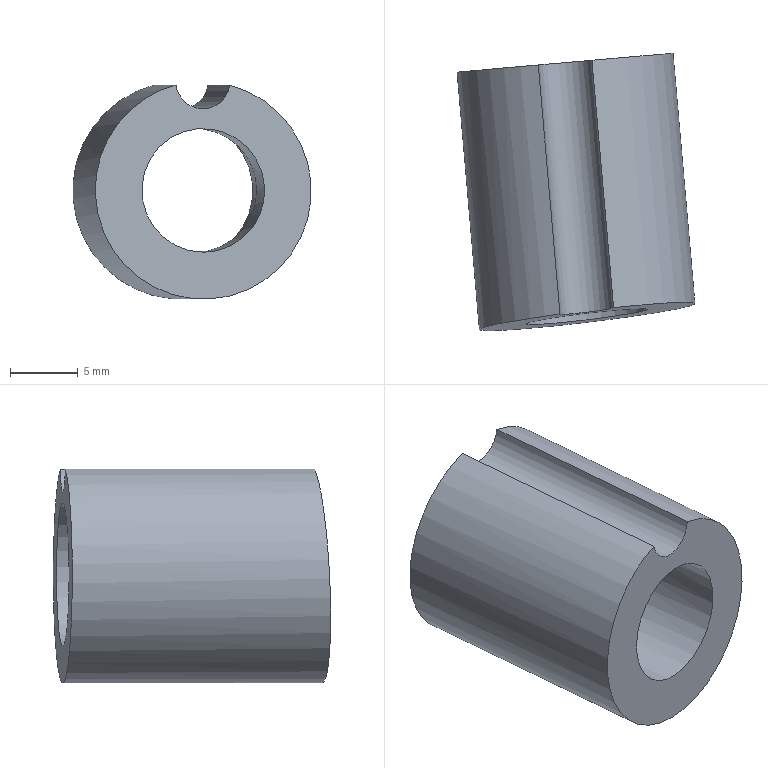Part | NX | features EKSD 16-20-9.100 2 | 1 solid | 7 faces | box 17.55 x 20.406 x 15.75 mm | volume 2161 mm3 | cylinder 4 | plane 3 | commonest cylinder face diameters 4 x1 9.1 x1 10.6 x1 16 x1
STEP:
#1=CARTESIAN_POINT('',(754.985,-30.446,-34.724));
#2=VERTEX_POINT('',#1);
#3=CARTESIAN_POINT('',(758.938,-30.1,-34.724));
#4=VERTEX_POINT('',#3);
#5=CARTESIAN_POINT('',(756.962,-30.273,-34.474));
#6=DIRECTION('',(0.08716,-0.9962,0.));
#7=DIRECTION('',(0.9962,0.08716,0.));
#8=AXIS2_PLACEMENT_3D('',#5,#6,#7);
#9=CIRCLE('',#8,2.);
#10=EDGE_CURVE('',#2,#4,#9,.T.);
#11=ORIENTED_EDGE('',*,*,#10,.T.);
#12=CARTESIAN_POINT('',(756.962,-30.273,-42.474));
#13=DIRECTION('',(0.08716,-0.9962,0.));
#14=DIRECTION('',(0.9962,0.08716,0.));
#15=AXIS2_PLACEMENT_3D('',#12,#13,#14);
#16=CIRCLE('',#15,8.);
#17=EDGE_CURVE('',#2,#4,#16,.T.);
#18=ORIENTED_EDGE('',*,*,#17,.F.);
#19=EDGE_LOOP('',(#11,#18));
#20=FACE_BOUND('',#19,.T.);
#21=CARTESIAN_POINT('',(751.682,-30.735,-42.474));
#22=VERTEX_POINT('',#21);
#23=CARTESIAN_POINT('',(756.962,-30.273,-42.474));
#24=DIRECTION('',(-0.08716,0.9962,0.));
#25=DIRECTION('',(-0.9962,-0.08716,0.));
#26=AXIS2_PLACEMENT_3D('',#23,#24,#25);
#27=CIRCLE('',#26,5.3);
#28=EDGE_CURVE('',#22,#22,#27,.T.);
#29=ORIENTED_EDGE('',*,*,#28,.F.);
#30=EDGE_LOOP('',(#29));
#31=FACE_BOUND('',#30,.T.);
#32=CARTESIAN_POINT('',(756.962,-30.273,-42.474));
#33=DIRECTION('',(-0.08716,0.9962,0.));
#34=DIRECTION('',(-0.9962,-0.08716,0.));
#35=AXIS2_PLACEMENT_3D('',#32,#33,#34);
#36=PLANE('',#35);
#37=ADVANCED_FACE('',(#20,#31),#36,.T.);
#38=CARTESIAN_POINT('',(760.531,-48.309,-34.724));
#39=VERTEX_POINT('',#38);
#40=CARTESIAN_POINT('',(756.589,-48.784,-34.724));
#41=VERTEX_POINT('',#40);
#42=CARTESIAN_POINT('',(758.559,-48.534,-34.474));
#43=DIRECTION('',(-0.1195,0.9915,-0.05097));
#44=DIRECTION('',(0.5313,0.1073,0.8404));
#45=AXIS2_PLACEMENT_3D('',#42,#43,#44);
#46=ELLIPSE('',#45,2.004,2.);
#47=EDGE_CURVE('',#39,#41,#46,.T.);
#48=ORIENTED_EDGE('',*,*,#47,.T.);
#49=CARTESIAN_POINT('',(758.595,-48.941,-42.474));
#50=DIRECTION('',(-0.1195,0.9915,-0.05097));
#51=DIRECTION('',(0.5313,0.1073,0.8404));
#52=AXIS2_PLACEMENT_3D('',#49,#50,#51);
#53=ELLIPSE('',#52,8.015,8.);
#54=EDGE_CURVE('',#39,#41,#53,.T.);
#55=ORIENTED_EDGE('',*,*,#54,.F.);
#56=EDGE_LOOP('',(#48,#55));
#57=FACE_BOUND('',#56,.T.);
#58=CARTESIAN_POINT('',(761.017,-48.452,-38.644));
#59=VERTEX_POINT('',#58);
#60=CARTESIAN_POINT('',(758.595,-48.941,-42.474));
#61=DIRECTION('',(-0.1195,0.9915,-0.05097));
#62=DIRECTION('',(0.5313,0.1073,0.8404));
#63=AXIS2_PLACEMENT_3D('',#60,#61,#62);
#64=ELLIPSE('',#63,4.558,4.55);
#65=EDGE_CURVE('',#59,#59,#64,.F.);
#66=ORIENTED_EDGE('',*,*,#65,.F.);
#67=EDGE_LOOP('',(#66));
#68=FACE_BOUND('',#67,.T.);
#69=CARTESIAN_POINT('',(707.484,-59.507,-128.15));
#70=DIRECTION('',(-0.1195,0.9915,-0.05097));
#71=DIRECTION('',(0.06611,0.05918,0.9961));
#72=AXIS2_PLACEMENT_3D('',#69,#70,#71);
#73=PLANE('',#72);
#74=ADVANCED_FACE('',(#57,#68),#73,.F.);
#75=CARTESIAN_POINT('',(759.81,-40.062,-34.724));
#76=DIRECTION('',(-0.08716,0.9962,0.));
#77=VECTOR('',#76,1000.);
#78=LINE('',#75,#77);
#79=EDGE_CURVE('',#39,#4,#78,.T.);
#80=ORIENTED_EDGE('',*,*,#79,.F.);
#81=ORIENTED_EDGE('',*,*,#54,.T.);
#82=CARTESIAN_POINT('',(755.856,-40.408,-34.724));
#83=DIRECTION('',(-0.08716,0.9962,0.));
#84=VECTOR('',#83,1000.);
#85=LINE('',#82,#84);
#86=EDGE_CURVE('',#2,#41,#85,.F.);
#87=ORIENTED_EDGE('',*,*,#86,.F.);
#88=ORIENTED_EDGE('',*,*,#17,.T.);
#89=EDGE_LOOP('',(#80,#81,#87,#88));
#90=FACE_BOUND('',#89,.T.);
#91=CARTESIAN_POINT('',(758.705,-50.197,-42.474));
#92=DIRECTION('',(-0.08716,0.9962,0.));
#93=DIRECTION('',(-0.9962,-0.08716,0.));
#94=AXIS2_PLACEMENT_3D('',#91,#92,#93);
#95=CYLINDRICAL_SURFACE('',#94,8.);
#96=ADVANCED_FACE('',(#90),#95,.T.);
#97=CARTESIAN_POINT('',(762.54,-41.831,-42.474));
#98=VERTEX_POINT('',#97);
#99=CARTESIAN_POINT('',(758.008,-42.228,-42.474));
#100=DIRECTION('',(0.08716,-0.9962,0.));
#101=DIRECTION('',(0.9962,0.08716,0.));
#102=AXIS2_PLACEMENT_3D('',#99,#100,#101);
#103=CIRCLE('',#102,4.55);
#104=EDGE_CURVE('',#98,#98,#103,.F.);
#105=ORIENTED_EDGE('',*,*,#104,.T.);
#106=EDGE_LOOP('',(#105));
#107=FACE_BOUND('',#106,.T.);
#108=ORIENTED_EDGE('',*,*,#65,.T.);
#109=EDGE_LOOP('',(#108));
#110=FACE_BOUND('',#109,.T.);
#111=CARTESIAN_POINT('',(758.792,-51.193,-42.474));
#112=DIRECTION('',(-0.08716,0.9962,0.));
#113=DIRECTION('',(-0.9962,-0.08716,0.));
#114=AXIS2_PLACEMENT_3D('',#111,#112,#113);
#115=CYLINDRICAL_SURFACE('',#114,4.55);
#116=ADVANCED_FACE('',(#107,#110),#115,.F.);
#117=CARTESIAN_POINT('',(752.728,-42.689,-42.474));
#118=VERTEX_POINT('',#117);
#119=CARTESIAN_POINT('',(758.008,-42.228,-42.474));
#120=DIRECTION('',(-0.08716,0.9962,0.));
#121=DIRECTION('',(-0.9962,-0.08716,0.));
#122=AXIS2_PLACEMENT_3D('',#119,#120,#121);
#123=CIRCLE('',#122,5.3);
#124=EDGE_CURVE('',#118,#118,#123,.T.);
#125=ORIENTED_EDGE('',*,*,#124,.T.);
#126=EDGE_LOOP('',(#125));
#127=FACE_BOUND('',#126,.T.);
#128=ORIENTED_EDGE('',*,*,#104,.F.);
#129=EDGE_LOOP('',(#128));
#130=FACE_BOUND('',#129,.T.);
#131=CARTESIAN_POINT('',(758.008,-42.228,-42.474));
#132=DIRECTION('',(0.08716,-0.9962,0.));
#133=DIRECTION('',(0.9962,0.08716,0.));
#134=AXIS2_PLACEMENT_3D('',#131,#132,#133);
#135=PLANE('',#134);
#136=ADVANCED_FACE('',(#127,#130),#135,.F.);
#137=ORIENTED_EDGE('',*,*,#28,.T.);
#138=EDGE_LOOP('',(#137));
#139=FACE_BOUND('',#138,.T.);
#140=ORIENTED_EDGE('',*,*,#124,.F.);
#141=EDGE_LOOP('',(#140));
#142=FACE_BOUND('',#141,.T.);
#143=CARTESIAN_POINT('',(758.008,-42.228,-42.474));
#144=DIRECTION('',(-0.08716,0.9962,0.));
#145=DIRECTION('',(-0.9962,-0.08716,0.));
#146=AXIS2_PLACEMENT_3D('',#143,#144,#145);
#147=CYLINDRICAL_SURFACE('',#146,5.3);
#148=ADVANCED_FACE('',(#139,#142),#147,.F.);
#149=ORIENTED_EDGE('',*,*,#79,.T.);
#150=ORIENTED_EDGE('',*,*,#10,.F.);
#151=ORIENTED_EDGE('',*,*,#86,.T.);
#152=ORIENTED_EDGE('',*,*,#47,.F.);
#153=EDGE_LOOP('',(#149,#150,#151,#152));
#154=FACE_BOUND('',#153,.T.);
#155=CARTESIAN_POINT('',(758.705,-50.197,-34.474));
#156=DIRECTION('',(-0.08716,0.9962,0.));
#157=DIRECTION('',(-0.9962,-0.08716,0.));
#158=AXIS2_PLACEMENT_3D('',#155,#156,#157);
#159=CYLINDRICAL_SURFACE('',#158,2.);
#160=ADVANCED_FACE('',(#154),#159,.F.);
#161=CLOSED_SHELL('',(#37,#74,#96,#116,#136,#148,#160));
#162=MANIFOLD_SOLID_BREP('',#161);
#163=(LENGTH_UNIT()NAMED_UNIT(*)SI_UNIT(.MILLI.,.METRE.));
#164=UNCERTAINTY_MEASURE_WITH_UNIT(LENGTH_MEASURE(0.00001),#163,'','');
#165=(NAMED_UNIT(*)PLANE_ANGLE_UNIT()SI_UNIT($,.RADIAN.));
#166=(NAMED_UNIT(*)SI_UNIT($,.STERADIAN.)SOLID_ANGLE_UNIT());
#167=(GEOMETRIC_REPRESENTATION_CONTEXT(3)GLOBAL_UNCERTAINTY_ASSIGNED_CONTEXT((#164))GLOBAL_UNIT_ASSIGNED_CONTEXT((#163,#165,#166))REPRESENTATION_CONTEXT('',''));
#168=ADVANCED_BREP_SHAPE_REPRESENTATION('',(#162),#167);